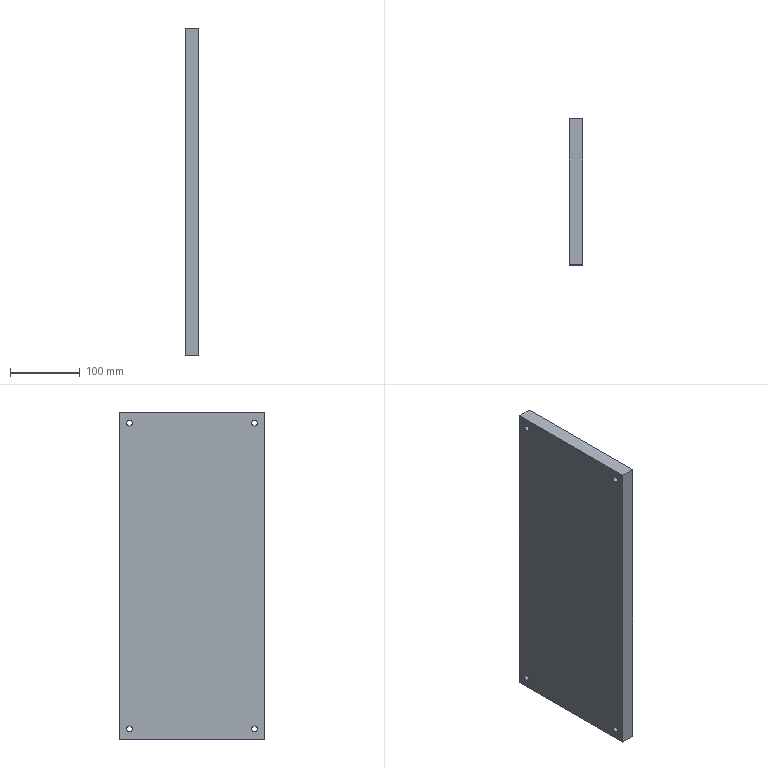Part | STEP file | A14-050 | 1 solid | 14 faces | box 20 x 210 x 470 mm | volume 1969460 mm3 | cylinder 8 | plane 6 | commonest cylinder face diameters 8.5 x8
STEP:
#1=CARTESIAN_POINT('',(0.,0.,0.));
#2=DIRECTION('',(0.,0.,1.));
#3=DIRECTION('',(1.,0.,0.));
#4=AXIS2_PLACEMENT_3D('',#1,#2,#3);
#5=CARTESIAN_POINT('',(-10.,90.,215.75));
#6=VERTEX_POINT('',#5);
#7=CARTESIAN_POINT('',(10.,90.,215.75));
#8=VERTEX_POINT('',#7);
#9=CARTESIAN_POINT('',(-10.,90.,215.75));
#10=DIRECTION('',(1.,0.,0.));
#11=VECTOR('',#10,1.);
#12=LINE('',#9,#11);
#13=CARTESIAN_POINT('',(-10.,90.,220.));
#14=DIRECTION('',(1.,0.,0.));
#15=DIRECTION('',(0.,0.,-1.));
#16=AXIS2_PLACEMENT_3D('',#13,#14,#15);
#17=CYLINDRICAL_SURFACE('',#16,4.25);
#18=CARTESIAN_POINT('',(6.283,0.));
#19=DIRECTION('',(0.,1.));
#20=VECTOR('',#19,1.);
#21=LINE('',#18,#20);
#22=(GEOMETRIC_REPRESENTATION_CONTEXT(2)PARAMETRIC_REPRESENTATION_CONTEXT()REPRESENTATION_CONTEXT('',''));
#23=DEFINITIONAL_REPRESENTATION('',(#21),#22);
#24=PCURVE('',#17,#23);
#25=CARTESIAN_POINT('',(-10.,90.,220.));
#26=DIRECTION('',(1.,0.,0.));
#27=DIRECTION('',(0.,0.,-1.));
#28=AXIS2_PLACEMENT_3D('',#25,#26,#27);
#29=CYLINDRICAL_SURFACE('',#28,4.25);
#30=CARTESIAN_POINT('',(0.,0.));
#31=DIRECTION('',(0.,1.));
#32=VECTOR('',#31,1.);
#33=LINE('',#30,#32);
#34=(GEOMETRIC_REPRESENTATION_CONTEXT(2)PARAMETRIC_REPRESENTATION_CONTEXT()REPRESENTATION_CONTEXT('',''));
#35=DEFINITIONAL_REPRESENTATION('',(#33),#34);
#36=PCURVE('',#29,#35);
#37=SURFACE_CURVE('',#12,(#24,#36),.PCURVE_S1.);
#38=EDGE_CURVE('',#6,#8,#37,.T.);
#39=ORIENTED_EDGE('',*,*,#38,.T.);
#40=CARTESIAN_POINT('',(10.,90.,224.25));
#41=VERTEX_POINT('',#40);
#42=CARTESIAN_POINT('',(10.,90.,220.));
#43=DIRECTION('',(1.,0.,0.));
#44=DIRECTION('',(0.,0.,-1.));
#45=AXIS2_PLACEMENT_3D('',#42,#43,#44);
#46=CIRCLE('',#45,4.25);
#47=CARTESIAN_POINT('',(0.,20.));
#48=DIRECTION('',(1.,0.));
#49=VECTOR('',#48,1.);
#50=LINE('',#47,#49);
#51=(GEOMETRIC_REPRESENTATION_CONTEXT(2)PARAMETRIC_REPRESENTATION_CONTEXT()REPRESENTATION_CONTEXT('',''));
#52=DEFINITIONAL_REPRESENTATION('',(#50),#51);
#53=PCURVE('',#17,#52);
#54=CARTESIAN_POINT('',(10.,0.,0.));
#55=DIRECTION('',(1.,0.,0.));
#56=DIRECTION('',(0.,0.,-1.));
#57=AXIS2_PLACEMENT_3D('',#54,#55,#56);
#58=PLANE('',#57);
#59=CARTESIAN_POINT('',(-220.,90.));
#60=DIRECTION('',(1.,0.));
#61=AXIS2_PLACEMENT_2D('',#59,#60);
#62=CIRCLE('',#61,4.25);
#63=(GEOMETRIC_REPRESENTATION_CONTEXT(2)PARAMETRIC_REPRESENTATION_CONTEXT()REPRESENTATION_CONTEXT('',''));
#64=DEFINITIONAL_REPRESENTATION('',(#62),#63);
#65=PCURVE('',#58,#64);
#66=SURFACE_CURVE('',#46,(#53,#65),.PCURVE_S1.);
#67=EDGE_CURVE('',#41,#8,#66,.T.);
#68=ORIENTED_EDGE('',*,*,#67,.F.);
#69=CARTESIAN_POINT('',(-10.,90.,224.25));
#70=VERTEX_POINT('',#69);
#71=CARTESIAN_POINT('',(-10.,90.,224.25));
#72=DIRECTION('',(1.,0.,0.));
#73=VECTOR('',#72,1.);
#74=LINE('',#71,#73);
#75=CARTESIAN_POINT('',(3.142,0.));
#76=DIRECTION('',(0.,1.));
#77=VECTOR('',#76,1.);
#78=LINE('',#75,#77);
#79=(GEOMETRIC_REPRESENTATION_CONTEXT(2)PARAMETRIC_REPRESENTATION_CONTEXT()REPRESENTATION_CONTEXT('',''));
#80=DEFINITIONAL_REPRESENTATION('',(#78),#79);
#81=PCURVE('',#17,#80);
#82=CARTESIAN_POINT('',(3.142,0.));
#83=DIRECTION('',(0.,1.));
#84=VECTOR('',#83,1.);
#85=LINE('',#82,#84);
#86=(GEOMETRIC_REPRESENTATION_CONTEXT(2)PARAMETRIC_REPRESENTATION_CONTEXT()REPRESENTATION_CONTEXT('',''));
#87=DEFINITIONAL_REPRESENTATION('',(#85),#86);
#88=PCURVE('',#29,#87);
#89=SURFACE_CURVE('',#74,(#81,#88),.PCURVE_S1.);
#90=EDGE_CURVE('',#70,#41,#89,.T.);
#91=ORIENTED_EDGE('',*,*,#90,.F.);
#92=CARTESIAN_POINT('',(-10.,90.,220.));
#93=DIRECTION('',(1.,0.,0.));
#94=DIRECTION('',(0.,0.,-1.));
#95=AXIS2_PLACEMENT_3D('',#92,#93,#94);
#96=CIRCLE('',#95,4.25);
#97=CARTESIAN_POINT('',(0.,0.));
#98=DIRECTION('',(1.,0.));
#99=VECTOR('',#98,1.);
#100=LINE('',#97,#99);
#101=(GEOMETRIC_REPRESENTATION_CONTEXT(2)PARAMETRIC_REPRESENTATION_CONTEXT()REPRESENTATION_CONTEXT('',''));
#102=DEFINITIONAL_REPRESENTATION('',(#100),#101);
#103=PCURVE('',#17,#102);
#104=CARTESIAN_POINT('',(-10.,0.,0.));
#105=DIRECTION('',(1.,0.,0.));
#106=DIRECTION('',(0.,0.,-1.));
#107=AXIS2_PLACEMENT_3D('',#104,#105,#106);
#108=PLANE('',#107);
#109=CARTESIAN_POINT('',(-220.,90.));
#110=DIRECTION('',(1.,0.));
#111=AXIS2_PLACEMENT_2D('',#109,#110);
#112=CIRCLE('',#111,4.25);
#113=(GEOMETRIC_REPRESENTATION_CONTEXT(2)PARAMETRIC_REPRESENTATION_CONTEXT()REPRESENTATION_CONTEXT('',''));
#114=DEFINITIONAL_REPRESENTATION('',(#112),#113);
#115=PCURVE('',#108,#114);
#116=SURFACE_CURVE('',#96,(#103,#115),.PCURVE_S1.);
#117=EDGE_CURVE('',#70,#6,#116,.T.);
#118=ORIENTED_EDGE('',*,*,#117,.T.);
#119=EDGE_LOOP('',(#39,#68,#91,#118));
#120=FACE_BOUND('',#119,.F.);
#121=ADVANCED_FACE('',(#120),#17,.F.);
#122=CARTESIAN_POINT('',(-10.,-90.,215.75));
#123=VERTEX_POINT('',#122);
#124=CARTESIAN_POINT('',(10.,-90.,215.75));
#125=VERTEX_POINT('',#124);
#126=CARTESIAN_POINT('',(-10.,-90.,215.75));
#127=DIRECTION('',(1.,0.,0.));
#128=VECTOR('',#127,1.);
#129=LINE('',#126,#128);
#130=CARTESIAN_POINT('',(-10.,-90.,220.));
#131=DIRECTION('',(1.,0.,0.));
#132=DIRECTION('',(0.,0.,-1.));
#133=AXIS2_PLACEMENT_3D('',#130,#131,#132);
#134=CYLINDRICAL_SURFACE('',#133,4.25);
#135=CARTESIAN_POINT('',(6.283,0.));
#136=DIRECTION('',(0.,1.));
#137=VECTOR('',#136,1.);
#138=LINE('',#135,#137);
#139=(GEOMETRIC_REPRESENTATION_CONTEXT(2)PARAMETRIC_REPRESENTATION_CONTEXT()REPRESENTATION_CONTEXT('',''));
#140=DEFINITIONAL_REPRESENTATION('',(#138),#139);
#141=PCURVE('',#134,#140);
#142=CARTESIAN_POINT('',(-10.,-90.,220.));
#143=DIRECTION('',(1.,0.,0.));
#144=DIRECTION('',(0.,0.,-1.));
#145=AXIS2_PLACEMENT_3D('',#142,#143,#144);
#146=CYLINDRICAL_SURFACE('',#145,4.25);
#147=CARTESIAN_POINT('',(0.,0.));
#148=DIRECTION('',(0.,1.));
#149=VECTOR('',#148,1.);
#150=LINE('',#147,#149);
#151=(GEOMETRIC_REPRESENTATION_CONTEXT(2)PARAMETRIC_REPRESENTATION_CONTEXT()REPRESENTATION_CONTEXT('',''));
#152=DEFINITIONAL_REPRESENTATION('',(#150),#151);
#153=PCURVE('',#146,#152);
#154=SURFACE_CURVE('',#129,(#141,#153),.PCURVE_S1.);
#155=EDGE_CURVE('',#123,#125,#154,.T.);
#156=ORIENTED_EDGE('',*,*,#155,.T.);
#157=CARTESIAN_POINT('',(10.,-90.,224.25));
#158=VERTEX_POINT('',#157);
#159=CARTESIAN_POINT('',(10.,-90.,220.));
#160=DIRECTION('',(1.,0.,0.));
#161=DIRECTION('',(0.,0.,-1.));
#162=AXIS2_PLACEMENT_3D('',#159,#160,#161);
#163=CIRCLE('',#162,4.25);
#164=CARTESIAN_POINT('',(0.,20.));
#165=DIRECTION('',(1.,0.));
#166=VECTOR('',#165,1.);
#167=LINE('',#164,#166);
#168=(GEOMETRIC_REPRESENTATION_CONTEXT(2)PARAMETRIC_REPRESENTATION_CONTEXT()REPRESENTATION_CONTEXT('',''));
#169=DEFINITIONAL_REPRESENTATION('',(#167),#168);
#170=PCURVE('',#134,#169);
#171=CARTESIAN_POINT('',(-220.,-90.));
#172=DIRECTION('',(1.,0.));
#173=AXIS2_PLACEMENT_2D('',#171,#172);
#174=CIRCLE('',#173,4.25);
#175=(GEOMETRIC_REPRESENTATION_CONTEXT(2)PARAMETRIC_REPRESENTATION_CONTEXT()REPRESENTATION_CONTEXT('',''));
#176=DEFINITIONAL_REPRESENTATION('',(#174),#175);
#177=PCURVE('',#58,#176);
#178=SURFACE_CURVE('',#163,(#170,#177),.PCURVE_S1.);
#179=EDGE_CURVE('',#158,#125,#178,.T.);
#180=ORIENTED_EDGE('',*,*,#179,.F.);
#181=CARTESIAN_POINT('',(-10.,-90.,224.25));
#182=VERTEX_POINT('',#181);
#183=CARTESIAN_POINT('',(-10.,-90.,224.25));
#184=DIRECTION('',(1.,0.,0.));
#185=VECTOR('',#184,1.);
#186=LINE('',#183,#185);
#187=CARTESIAN_POINT('',(3.142,0.));
#188=DIRECTION('',(0.,1.));
#189=VECTOR('',#188,1.);
#190=LINE('',#187,#189);
#191=(GEOMETRIC_REPRESENTATION_CONTEXT(2)PARAMETRIC_REPRESENTATION_CONTEXT()REPRESENTATION_CONTEXT('',''));
#192=DEFINITIONAL_REPRESENTATION('',(#190),#191);
#193=PCURVE('',#134,#192);
#194=CARTESIAN_POINT('',(3.142,0.));
#195=DIRECTION('',(0.,1.));
#196=VECTOR('',#195,1.);
#197=LINE('',#194,#196);
#198=(GEOMETRIC_REPRESENTATION_CONTEXT(2)PARAMETRIC_REPRESENTATION_CONTEXT()REPRESENTATION_CONTEXT('',''));
#199=DEFINITIONAL_REPRESENTATION('',(#197),#198);
#200=PCURVE('',#146,#199);
#201=SURFACE_CURVE('',#186,(#193,#200),.PCURVE_S1.);
#202=EDGE_CURVE('',#182,#158,#201,.T.);
#203=ORIENTED_EDGE('',*,*,#202,.F.);
#204=CARTESIAN_POINT('',(-10.,-90.,220.));
#205=DIRECTION('',(1.,0.,0.));
#206=DIRECTION('',(0.,0.,-1.));
#207=AXIS2_PLACEMENT_3D('',#204,#205,#206);
#208=CIRCLE('',#207,4.25);
#209=CARTESIAN_POINT('',(0.,0.));
#210=DIRECTION('',(1.,0.));
#211=VECTOR('',#210,1.);
#212=LINE('',#209,#211);
#213=(GEOMETRIC_REPRESENTATION_CONTEXT(2)PARAMETRIC_REPRESENTATION_CONTEXT()REPRESENTATION_CONTEXT('',''));
#214=DEFINITIONAL_REPRESENTATION('',(#212),#213);
#215=PCURVE('',#134,#214);
#216=CARTESIAN_POINT('',(-220.,-90.));
#217=DIRECTION('',(1.,0.));
#218=AXIS2_PLACEMENT_2D('',#216,#217);
#219=CIRCLE('',#218,4.25);
#220=(GEOMETRIC_REPRESENTATION_CONTEXT(2)PARAMETRIC_REPRESENTATION_CONTEXT()REPRESENTATION_CONTEXT('',''));
#221=DEFINITIONAL_REPRESENTATION('',(#219),#220);
#222=PCURVE('',#108,#221);
#223=SURFACE_CURVE('',#208,(#215,#222),.PCURVE_S1.);
#224=EDGE_CURVE('',#182,#123,#223,.T.);
#225=ORIENTED_EDGE('',*,*,#224,.T.);
#226=EDGE_LOOP('',(#156,#180,#203,#225));
#227=FACE_BOUND('',#226,.F.);
#228=ADVANCED_FACE('',(#227),#134,.F.);
#229=CARTESIAN_POINT('',(-10.,-90.,-224.25));
#230=VERTEX_POINT('',#229);
#231=CARTESIAN_POINT('',(10.,-90.,-224.25));
#232=VERTEX_POINT('',#231);
#233=CARTESIAN_POINT('',(-10.,-90.,-224.25));
#234=DIRECTION('',(1.,0.,0.));
#235=VECTOR('',#234,1.);
#236=LINE('',#233,#235);
#237=CARTESIAN_POINT('',(-10.,-90.,-220.));
#238=DIRECTION('',(1.,0.,0.));
#239=DIRECTION('',(0.,0.,-1.));
#240=AXIS2_PLACEMENT_3D('',#237,#238,#239);
#241=CYLINDRICAL_SURFACE('',#240,4.25);
#242=CARTESIAN_POINT('',(6.283,0.));
#243=DIRECTION('',(0.,1.));
#244=VECTOR('',#243,1.);
#245=LINE('',#242,#244);
#246=(GEOMETRIC_REPRESENTATION_CONTEXT(2)PARAMETRIC_REPRESENTATION_CONTEXT()REPRESENTATION_CONTEXT('',''));
#247=DEFINITIONAL_REPRESENTATION('',(#245),#246);
#248=PCURVE('',#241,#247);
#249=CARTESIAN_POINT('',(-10.,-90.,-220.));
#250=DIRECTION('',(1.,0.,0.));
#251=DIRECTION('',(0.,0.,-1.));
#252=AXIS2_PLACEMENT_3D('',#249,#250,#251);
#253=CYLINDRICAL_SURFACE('',#252,4.25);
#254=CARTESIAN_POINT('',(0.,0.));
#255=DIRECTION('',(0.,1.));
#256=VECTOR('',#255,1.);
#257=LINE('',#254,#256);
#258=(GEOMETRIC_REPRESENTATION_CONTEXT(2)PARAMETRIC_REPRESENTATION_CONTEXT()REPRESENTATION_CONTEXT('',''));
#259=DEFINITIONAL_REPRESENTATION('',(#257),#258);
#260=PCURVE('',#253,#259);
#261=SURFACE_CURVE('',#236,(#248,#260),.PCURVE_S1.);
#262=EDGE_CURVE('',#230,#232,#261,.T.);
#263=ORIENTED_EDGE('',*,*,#262,.T.);
#264=CARTESIAN_POINT('',(10.,-90.,-215.75));
#265=VERTEX_POINT('',#264);
#266=CARTESIAN_POINT('',(10.,-90.,-220.));
#267=DIRECTION('',(1.,0.,0.));
#268=DIRECTION('',(0.,0.,-1.));
#269=AXIS2_PLACEMENT_3D('',#266,#267,#268);
#270=CIRCLE('',#269,4.25);
#271=CARTESIAN_POINT('',(0.,20.));
#272=DIRECTION('',(1.,0.));
#273=VECTOR('',#272,1.);
#274=LINE('',#271,#273);
#275=(GEOMETRIC_REPRESENTATION_CONTEXT(2)PARAMETRIC_REPRESENTATION_CONTEXT()REPRESENTATION_CONTEXT('',''));
#276=DEFINITIONAL_REPRESENTATION('',(#274),#275);
#277=PCURVE('',#241,#276);
#278=CARTESIAN_POINT('',(220.,-90.));
#279=DIRECTION('',(1.,0.));
#280=AXIS2_PLACEMENT_2D('',#278,#279);
#281=CIRCLE('',#280,4.25);
#282=(GEOMETRIC_REPRESENTATION_CONTEXT(2)PARAMETRIC_REPRESENTATION_CONTEXT()REPRESENTATION_CONTEXT('',''));
#283=DEFINITIONAL_REPRESENTATION('',(#281),#282);
#284=PCURVE('',#58,#283);
#285=SURFACE_CURVE('',#270,(#277,#284),.PCURVE_S1.);
#286=EDGE_CURVE('',#265,#232,#285,.T.);
#287=ORIENTED_EDGE('',*,*,#286,.F.);
#288=CARTESIAN_POINT('',(-10.,-90.,-215.75));
#289=VERTEX_POINT('',#288);
#290=CARTESIAN_POINT('',(-10.,-90.,-215.75));
#291=DIRECTION('',(1.,0.,0.));
#292=VECTOR('',#291,1.);
#293=LINE('',#290,#292);
#294=CARTESIAN_POINT('',(3.142,0.));
#295=DIRECTION('',(0.,1.));
#296=VECTOR('',#295,1.);
#297=LINE('',#294,#296);
#298=(GEOMETRIC_REPRESENTATION_CONTEXT(2)PARAMETRIC_REPRESENTATION_CONTEXT()REPRESENTATION_CONTEXT('',''));
#299=DEFINITIONAL_REPRESENTATION('',(#297),#298);
#300=PCURVE('',#241,#299);
#301=CARTESIAN_POINT('',(3.142,0.));
#302=DIRECTION('',(0.,1.));
#303=VECTOR('',#302,1.);
#304=LINE('',#301,#303);
#305=(GEOMETRIC_REPRESENTATION_CONTEXT(2)PARAMETRIC_REPRESENTATION_CONTEXT()REPRESENTATION_CONTEXT('',''));
#306=DEFINITIONAL_REPRESENTATION('',(#304),#305);
#307=PCURVE('',#253,#306);
#308=SURFACE_CURVE('',#293,(#300,#307),.PCURVE_S1.);
#309=EDGE_CURVE('',#289,#265,#308,.T.);
#310=ORIENTED_EDGE('',*,*,#309,.F.);
#311=CARTESIAN_POINT('',(-10.,-90.,-220.));
#312=DIRECTION('',(1.,0.,0.));
#313=DIRECTION('',(0.,0.,-1.));
#314=AXIS2_PLACEMENT_3D('',#311,#312,#313);
#315=CIRCLE('',#314,4.25);
#316=CARTESIAN_POINT('',(0.,0.));
#317=DIRECTION('',(1.,0.));
#318=VECTOR('',#317,1.);
#319=LINE('',#316,#318);
#320=(GEOMETRIC_REPRESENTATION_CONTEXT(2)PARAMETRIC_REPRESENTATION_CONTEXT()REPRESENTATION_CONTEXT('',''));
#321=DEFINITIONAL_REPRESENTATION('',(#319),#320);
#322=PCURVE('',#241,#321);
#323=CARTESIAN_POINT('',(220.,-90.));
#324=DIRECTION('',(1.,0.));
#325=AXIS2_PLACEMENT_2D('',#323,#324);
#326=CIRCLE('',#325,4.25);
#327=(GEOMETRIC_REPRESENTATION_CONTEXT(2)PARAMETRIC_REPRESENTATION_CONTEXT()REPRESENTATION_CONTEXT('',''));
#328=DEFINITIONAL_REPRESENTATION('',(#326),#327);
#329=PCURVE('',#108,#328);
#330=SURFACE_CURVE('',#315,(#322,#329),.PCURVE_S1.);
#331=EDGE_CURVE('',#289,#230,#330,.T.);
#332=ORIENTED_EDGE('',*,*,#331,.T.);
#333=EDGE_LOOP('',(#263,#287,#310,#332));
#334=FACE_BOUND('',#333,.F.);
#335=ADVANCED_FACE('',(#334),#241,.F.);
#336=CARTESIAN_POINT('',(-10.,90.,-224.25));
#337=VERTEX_POINT('',#336);
#338=CARTESIAN_POINT('',(10.,90.,-224.25));
#339=VERTEX_POINT('',#338);
#340=CARTESIAN_POINT('',(-10.,90.,-224.25));
#341=DIRECTION('',(1.,0.,0.));
#342=VECTOR('',#341,1.);
#343=LINE('',#340,#342);
#344=CARTESIAN_POINT('',(-10.,90.,-220.));
#345=DIRECTION('',(1.,0.,0.));
#346=DIRECTION('',(0.,0.,-1.));
#347=AXIS2_PLACEMENT_3D('',#344,#345,#346);
#348=CYLINDRICAL_SURFACE('',#347,4.25);
#349=CARTESIAN_POINT('',(6.283,0.));
#350=DIRECTION('',(0.,1.));
#351=VECTOR('',#350,1.);
#352=LINE('',#349,#351);
#353=(GEOMETRIC_REPRESENTATION_CONTEXT(2)PARAMETRIC_REPRESENTATION_CONTEXT()REPRESENTATION_CONTEXT('',''));
#354=DEFINITIONAL_REPRESENTATION('',(#352),#353);
#355=PCURVE('',#348,#354);
#356=CARTESIAN_POINT('',(-10.,90.,-220.));
#357=DIRECTION('',(1.,0.,0.));
#358=DIRECTION('',(0.,0.,-1.));
#359=AXIS2_PLACEMENT_3D('',#356,#357,#358);
#360=CYLINDRICAL_SURFACE('',#359,4.25);
#361=CARTESIAN_POINT('',(0.,0.));
#362=DIRECTION('',(0.,1.));
#363=VECTOR('',#362,1.);
#364=LINE('',#361,#363);
#365=(GEOMETRIC_REPRESENTATION_CONTEXT(2)PARAMETRIC_REPRESENTATION_CONTEXT()REPRESENTATION_CONTEXT('',''));
#366=DEFINITIONAL_REPRESENTATION('',(#364),#365);
#367=PCURVE('',#360,#366);
#368=SURFACE_CURVE('',#343,(#355,#367),.PCURVE_S1.);
#369=EDGE_CURVE('',#337,#339,#368,.T.);
#370=ORIENTED_EDGE('',*,*,#369,.T.);
#371=CARTESIAN_POINT('',(10.,90.,-215.75));
#372=VERTEX_POINT('',#371);
#373=CARTESIAN_POINT('',(10.,90.,-220.));
#374=DIRECTION('',(1.,0.,0.));
#375=DIRECTION('',(0.,0.,-1.));
#376=AXIS2_PLACEMENT_3D('',#373,#374,#375);
#377=CIRCLE('',#376,4.25);
#378=CARTESIAN_POINT('',(0.,20.));
#379=DIRECTION('',(1.,0.));
#380=VECTOR('',#379,1.);
#381=LINE('',#378,#380);
#382=(GEOMETRIC_REPRESENTATION_CONTEXT(2)PARAMETRIC_REPRESENTATION_CONTEXT()REPRESENTATION_CONTEXT('',''));
#383=DEFINITIONAL_REPRESENTATION('',(#381),#382);
#384=PCURVE('',#348,#383);
#385=CARTESIAN_POINT('',(220.,90.));
#386=DIRECTION('',(1.,0.));
#387=AXIS2_PLACEMENT_2D('',#385,#386);
#388=CIRCLE('',#387,4.25);
#389=(GEOMETRIC_REPRESENTATION_CONTEXT(2)PARAMETRIC_REPRESENTATION_CONTEXT()REPRESENTATION_CONTEXT('',''));
#390=DEFINITIONAL_REPRESENTATION('',(#388),#389);
#391=PCURVE('',#58,#390);
#392=SURFACE_CURVE('',#377,(#384,#391),.PCURVE_S1.);
#393=EDGE_CURVE('',#372,#339,#392,.T.);
#394=ORIENTED_EDGE('',*,*,#393,.F.);
#395=CARTESIAN_POINT('',(-10.,90.,-215.75));
#396=VERTEX_POINT('',#395);
#397=CARTESIAN_POINT('',(-10.,90.,-215.75));
#398=DIRECTION('',(1.,0.,0.));
#399=VECTOR('',#398,1.);
#400=LINE('',#397,#399);
#401=CARTESIAN_POINT('',(3.142,0.));
#402=DIRECTION('',(0.,1.));
#403=VECTOR('',#402,1.);
#404=LINE('',#401,#403);
#405=(GEOMETRIC_REPRESENTATION_CONTEXT(2)PARAMETRIC_REPRESENTATION_CONTEXT()REPRESENTATION_CONTEXT('',''));
#406=DEFINITIONAL_REPRESENTATION('',(#404),#405);
#407=PCURVE('',#348,#406);
#408=CARTESIAN_POINT('',(3.142,0.));
#409=DIRECTION('',(0.,1.));
#410=VECTOR('',#409,1.);
#411=LINE('',#408,#410);
#412=(GEOMETRIC_REPRESENTATION_CONTEXT(2)PARAMETRIC_REPRESENTATION_CONTEXT()REPRESENTATION_CONTEXT('',''));
#413=DEFINITIONAL_REPRESENTATION('',(#411),#412);
#414=PCURVE('',#360,#413);
#415=SURFACE_CURVE('',#400,(#407,#414),.PCURVE_S1.);
#416=EDGE_CURVE('',#396,#372,#415,.T.);
#417=ORIENTED_EDGE('',*,*,#416,.F.);
#418=CARTESIAN_POINT('',(-10.,90.,-220.));
#419=DIRECTION('',(1.,0.,0.));
#420=DIRECTION('',(0.,0.,-1.));
#421=AXIS2_PLACEMENT_3D('',#418,#419,#420);
#422=CIRCLE('',#421,4.25);
#423=CARTESIAN_POINT('',(0.,0.));
#424=DIRECTION('',(1.,0.));
#425=VECTOR('',#424,1.);
#426=LINE('',#423,#425);
#427=(GEOMETRIC_REPRESENTATION_CONTEXT(2)PARAMETRIC_REPRESENTATION_CONTEXT()REPRESENTATION_CONTEXT('',''));
#428=DEFINITIONAL_REPRESENTATION('',(#426),#427);
#429=PCURVE('',#348,#428);
#430=CARTESIAN_POINT('',(220.,90.));
#431=DIRECTION('',(1.,0.));
#432=AXIS2_PLACEMENT_2D('',#430,#431);
#433=CIRCLE('',#432,4.25);
#434=(GEOMETRIC_REPRESENTATION_CONTEXT(2)PARAMETRIC_REPRESENTATION_CONTEXT()REPRESENTATION_CONTEXT('',''));
#435=DEFINITIONAL_REPRESENTATION('',(#433),#434);
#436=PCURVE('',#108,#435);
#437=SURFACE_CURVE('',#422,(#429,#436),.PCURVE_S1.);
#438=EDGE_CURVE('',#396,#337,#437,.T.);
#439=ORIENTED_EDGE('',*,*,#438,.T.);
#440=EDGE_LOOP('',(#370,#394,#417,#439));
#441=FACE_BOUND('',#440,.F.);
#442=ADVANCED_FACE('',(#441),#348,.F.);
#443=CARTESIAN_POINT('',(-10.,-105.,-235.));
#444=VERTEX_POINT('',#443);
#445=CARTESIAN_POINT('',(-10.,105.,-235.));
#446=VERTEX_POINT('',#445);
#447=CARTESIAN_POINT('',(-10.,105.,-235.));
#448=DIRECTION('',(0.,1.,0.));
#449=VECTOR('',#448,1.);
#450=LINE('',#447,#449);
#451=CARTESIAN_POINT('',(10.,105.,-235.));
#452=DIRECTION('',(0.,0.,1.));
#453=DIRECTION('',(1.,0.,0.));
#454=AXIS2_PLACEMENT_3D('',#451,#452,#453);
#455=PLANE('',#454);
#456=CARTESIAN_POINT('',(-20.,0.));
#457=DIRECTION('',(0.,1.));
#458=VECTOR('',#457,1.);
#459=LINE('',#456,#458);
#460=(GEOMETRIC_REPRESENTATION_CONTEXT(2)PARAMETRIC_REPRESENTATION_CONTEXT()REPRESENTATION_CONTEXT('',''));
#461=DEFINITIONAL_REPRESENTATION('',(#459),#460);
#462=PCURVE('',#455,#461);
#463=CARTESIAN_POINT('',(235.,105.));
#464=DIRECTION('',(0.,1.));
#465=VECTOR('',#464,1.);
#466=LINE('',#463,#465);
#467=(GEOMETRIC_REPRESENTATION_CONTEXT(2)PARAMETRIC_REPRESENTATION_CONTEXT()REPRESENTATION_CONTEXT('',''));
#468=DEFINITIONAL_REPRESENTATION('',(#466),#467);
#469=PCURVE('',#108,#468);
#470=SURFACE_CURVE('',#450,(#462,#469),.PCURVE_S1.);
#471=EDGE_CURVE('',#444,#446,#470,.T.);
#472=ORIENTED_EDGE('',*,*,#471,.T.);
#473=CARTESIAN_POINT('',(10.,105.,-235.));
#474=VERTEX_POINT('',#473);
#475=CARTESIAN_POINT('',(10.,105.,-235.));
#476=DIRECTION('',(-1.,0.,0.));
#477=VECTOR('',#476,1.);
#478=LINE('',#475,#477);
#479=CARTESIAN_POINT('',(0.,0.));
#480=DIRECTION('',(-1.,0.));
#481=VECTOR('',#480,1.);
#482=LINE('',#479,#481);
#483=(GEOMETRIC_REPRESENTATION_CONTEXT(2)PARAMETRIC_REPRESENTATION_CONTEXT()REPRESENTATION_CONTEXT('',''));
#484=DEFINITIONAL_REPRESENTATION('',(#482),#483);
#485=PCURVE('',#455,#484);
#486=CARTESIAN_POINT('',(10.,105.,235.));
#487=DIRECTION('',(0.,-1.,0.));
#488=DIRECTION('',(0.,0.,-1.));
#489=AXIS2_PLACEMENT_3D('',#486,#487,#488);
#490=PLANE('',#489);
#491=CARTESIAN_POINT('',(470.,0.));
#492=DIRECTION('',(0.,-1.));
#493=VECTOR('',#492,1.);
#494=LINE('',#491,#493);
#495=(GEOMETRIC_REPRESENTATION_CONTEXT(2)PARAMETRIC_REPRESENTATION_CONTEXT()REPRESENTATION_CONTEXT('',''));
#496=DEFINITIONAL_REPRESENTATION('',(#494),#495);
#497=PCURVE('',#490,#496);
#498=SURFACE_CURVE('',#478,(#485,#497),.PCURVE_S1.);
#499=EDGE_CURVE('',#474,#446,#498,.T.);
#500=ORIENTED_EDGE('',*,*,#499,.F.);
#501=CARTESIAN_POINT('',(10.,-105.,-235.));
#502=VERTEX_POINT('',#501);
#503=CARTESIAN_POINT('',(10.,105.,-235.));
#504=DIRECTION('',(0.,1.,0.));
#505=VECTOR('',#504,1.);
#506=LINE('',#503,#505);
#507=CARTESIAN_POINT('',(0.,0.));
#508=DIRECTION('',(0.,1.));
#509=VECTOR('',#508,1.);
#510=LINE('',#507,#509);
#511=(GEOMETRIC_REPRESENTATION_CONTEXT(2)PARAMETRIC_REPRESENTATION_CONTEXT()REPRESENTATION_CONTEXT('',''));
#512=DEFINITIONAL_REPRESENTATION('',(#510),#511);
#513=PCURVE('',#455,#512);
#514=CARTESIAN_POINT('',(235.,105.));
#515=DIRECTION('',(0.,1.));
#516=VECTOR('',#515,1.);
#517=LINE('',#514,#516);
#518=(GEOMETRIC_REPRESENTATION_CONTEXT(2)PARAMETRIC_REPRESENTATION_CONTEXT()REPRESENTATION_CONTEXT('',''));
#519=DEFINITIONAL_REPRESENTATION('',(#517),#518);
#520=PCURVE('',#58,#519);
#521=SURFACE_CURVE('',#506,(#513,#520),.PCURVE_S1.);
#522=EDGE_CURVE('',#502,#474,#521,.T.);
#523=ORIENTED_EDGE('',*,*,#522,.F.);
#524=CARTESIAN_POINT('',(10.,-105.,-235.));
#525=DIRECTION('',(-1.,0.,0.));
#526=VECTOR('',#525,1.);
#527=LINE('',#524,#526);
#528=CARTESIAN_POINT('',(0.,-210.));
#529=DIRECTION('',(-1.,0.));
#530=VECTOR('',#529,1.);
#531=LINE('',#528,#530);
#532=(GEOMETRIC_REPRESENTATION_CONTEXT(2)PARAMETRIC_REPRESENTATION_CONTEXT()REPRESENTATION_CONTEXT('',''));
#533=DEFINITIONAL_REPRESENTATION('',(#531),#532);
#534=PCURVE('',#455,#533);
#535=CARTESIAN_POINT('',(10.,-105.,235.));
#536=DIRECTION('',(0.,1.,0.));
#537=DIRECTION('',(0.,0.,1.));
#538=AXIS2_PLACEMENT_3D('',#535,#536,#537);
#539=PLANE('',#538);
#540=CARTESIAN_POINT('',(-470.,0.));
#541=DIRECTION('',(0.,-1.));
#542=VECTOR('',#541,1.);
#543=LINE('',#540,#542);
#544=(GEOMETRIC_REPRESENTATION_CONTEXT(2)PARAMETRIC_REPRESENTATION_CONTEXT()REPRESENTATION_CONTEXT('',''));
#545=DEFINITIONAL_REPRESENTATION('',(#543),#544);
#546=PCURVE('',#539,#545);
#547=SURFACE_CURVE('',#527,(#534,#546),.PCURVE_S1.);
#548=EDGE_CURVE('',#502,#444,#547,.T.);
#549=ORIENTED_EDGE('',*,*,#548,.T.);
#550=EDGE_LOOP('',(#472,#500,#523,#549));
#551=FACE_BOUND('',#550,.T.);
#552=ADVANCED_FACE('',(#551),#455,.F.);
#553=CARTESIAN_POINT('',(-10.,105.,235.));
#554=VERTEX_POINT('',#553);
#555=CARTESIAN_POINT('',(-10.,105.,235.));
#556=DIRECTION('',(0.,0.,1.));
#557=VECTOR('',#556,1.);
#558=LINE('',#555,#557);
#559=CARTESIAN_POINT('',(0.,-20.));
#560=DIRECTION('',(-1.,0.));
#561=VECTOR('',#560,1.);
#562=LINE('',#559,#561);
#563=(GEOMETRIC_REPRESENTATION_CONTEXT(2)PARAMETRIC_REPRESENTATION_CONTEXT()REPRESENTATION_CONTEXT('',''));
#564=DEFINITIONAL_REPRESENTATION('',(#562),#563);
#565=PCURVE('',#490,#564);
#566=CARTESIAN_POINT('',(-235.,105.));
#567=DIRECTION('',(-1.,0.));
#568=VECTOR('',#567,1.);
#569=LINE('',#566,#568);
#570=(GEOMETRIC_REPRESENTATION_CONTEXT(2)PARAMETRIC_REPRESENTATION_CONTEXT()REPRESENTATION_CONTEXT('',''));
#571=DEFINITIONAL_REPRESENTATION('',(#569),#570);
#572=PCURVE('',#108,#571);
#573=SURFACE_CURVE('',#558,(#565,#572),.PCURVE_S1.);
#574=EDGE_CURVE('',#446,#554,#573,.T.);
#575=ORIENTED_EDGE('',*,*,#574,.T.);
#576=CARTESIAN_POINT('',(10.,105.,235.));
#577=VERTEX_POINT('',#576);
#578=CARTESIAN_POINT('',(10.,105.,235.));
#579=DIRECTION('',(-1.,0.,0.));
#580=VECTOR('',#579,1.);
#581=LINE('',#578,#580);
#582=CARTESIAN_POINT('',(0.,0.));
#583=DIRECTION('',(0.,-1.));
#584=VECTOR('',#583,1.);
#585=LINE('',#582,#584);
#586=(GEOMETRIC_REPRESENTATION_CONTEXT(2)PARAMETRIC_REPRESENTATION_CONTEXT()REPRESENTATION_CONTEXT('',''));
#587=DEFINITIONAL_REPRESENTATION('',(#585),#586);
#588=PCURVE('',#490,#587);
#589=CARTESIAN_POINT('',(10.,105.,235.));
#590=DIRECTION('',(0.,0.,-1.));
#591=DIRECTION('',(-1.,0.,0.));
#592=AXIS2_PLACEMENT_3D('',#589,#590,#591);
#593=PLANE('',#592);
#594=CARTESIAN_POINT('',(0.,0.));
#595=DIRECTION('',(1.,0.));
#596=VECTOR('',#595,1.);
#597=LINE('',#594,#596);
#598=(GEOMETRIC_REPRESENTATION_CONTEXT(2)PARAMETRIC_REPRESENTATION_CONTEXT()REPRESENTATION_CONTEXT('',''));
#599=DEFINITIONAL_REPRESENTATION('',(#597),#598);
#600=PCURVE('',#593,#599);
#601=SURFACE_CURVE('',#581,(#588,#600),.PCURVE_S1.);
#602=EDGE_CURVE('',#577,#554,#601,.T.);
#603=ORIENTED_EDGE('',*,*,#602,.F.);
#604=CARTESIAN_POINT('',(10.,105.,235.));
#605=DIRECTION('',(0.,0.,1.));
#606=VECTOR('',#605,1.);
#607=LINE('',#604,#606);
#608=CARTESIAN_POINT('',(0.,0.));
#609=DIRECTION('',(-1.,0.));
#610=VECTOR('',#609,1.);
#611=LINE('',#608,#610);
#612=(GEOMETRIC_REPRESENTATION_CONTEXT(2)PARAMETRIC_REPRESENTATION_CONTEXT()REPRESENTATION_CONTEXT('',''));
#613=DEFINITIONAL_REPRESENTATION('',(#611),#612);
#614=PCURVE('',#490,#613);
#615=CARTESIAN_POINT('',(-235.,105.));
#616=DIRECTION('',(-1.,0.));
#617=VECTOR('',#616,1.);
#618=LINE('',#615,#617);
#619=(GEOMETRIC_REPRESENTATION_CONTEXT(2)PARAMETRIC_REPRESENTATION_CONTEXT()REPRESENTATION_CONTEXT('',''));
#620=DEFINITIONAL_REPRESENTATION('',(#618),#619);
#621=PCURVE('',#58,#620);
#622=SURFACE_CURVE('',#607,(#614,#621),.PCURVE_S1.);
#623=EDGE_CURVE('',#474,#577,#622,.T.);
#624=ORIENTED_EDGE('',*,*,#623,.F.);
#625=ORIENTED_EDGE('',*,*,#499,.T.);
#626=EDGE_LOOP('',(#575,#603,#624,#625));
#627=FACE_BOUND('',#626,.T.);
#628=ADVANCED_FACE('',(#627),#490,.F.);
#629=CARTESIAN_POINT('',(-10.,-105.,235.));
#630=VERTEX_POINT('',#629);
#631=CARTESIAN_POINT('',(-10.,105.,235.));
#632=DIRECTION('',(0.,-1.,0.));
#633=VECTOR('',#632,1.);
#634=LINE('',#631,#633);
#635=CARTESIAN_POINT('',(20.,0.));
#636=DIRECTION('',(0.,-1.));
#637=VECTOR('',#636,1.);
#638=LINE('',#635,#637);
#639=(GEOMETRIC_REPRESENTATION_CONTEXT(2)PARAMETRIC_REPRESENTATION_CONTEXT()REPRESENTATION_CONTEXT('',''));
#640=DEFINITIONAL_REPRESENTATION('',(#638),#639);
#641=PCURVE('',#593,#640);
#642=CARTESIAN_POINT('',(-235.,105.));
#643=DIRECTION('',(0.,-1.));
#644=VECTOR('',#643,1.);
#645=LINE('',#642,#644);
#646=(GEOMETRIC_REPRESENTATION_CONTEXT(2)PARAMETRIC_REPRESENTATION_CONTEXT()REPRESENTATION_CONTEXT('',''));
#647=DEFINITIONAL_REPRESENTATION('',(#645),#646);
#648=PCURVE('',#108,#647);
#649=SURFACE_CURVE('',#634,(#641,#648),.PCURVE_S1.);
#650=EDGE_CURVE('',#554,#630,#649,.T.);
#651=ORIENTED_EDGE('',*,*,#650,.T.);
#652=CARTESIAN_POINT('',(10.,-105.,235.));
#653=VERTEX_POINT('',#652);
#654=CARTESIAN_POINT('',(10.,-105.,235.));
#655=DIRECTION('',(-1.,0.,0.));
#656=VECTOR('',#655,1.);
#657=LINE('',#654,#656);
#658=CARTESIAN_POINT('',(0.,-210.));
#659=DIRECTION('',(1.,0.));
#660=VECTOR('',#659,1.);
#661=LINE('',#658,#660);
#662=(GEOMETRIC_REPRESENTATION_CONTEXT(2)PARAMETRIC_REPRESENTATION_CONTEXT()REPRESENTATION_CONTEXT('',''));
#663=DEFINITIONAL_REPRESENTATION('',(#661),#662);
#664=PCURVE('',#593,#663);
#665=CARTESIAN_POINT('',(0.,0.));
#666=DIRECTION('',(0.,-1.));
#667=VECTOR('',#666,1.);
#668=LINE('',#665,#667);
#669=(GEOMETRIC_REPRESENTATION_CONTEXT(2)PARAMETRIC_REPRESENTATION_CONTEXT()REPRESENTATION_CONTEXT('',''));
#670=DEFINITIONAL_REPRESENTATION('',(#668),#669);
#671=PCURVE('',#539,#670);
#672=SURFACE_CURVE('',#657,(#664,#671),.PCURVE_S1.);
#673=EDGE_CURVE('',#653,#630,#672,.T.);
#674=ORIENTED_EDGE('',*,*,#673,.F.);
#675=CARTESIAN_POINT('',(10.,105.,235.));
#676=DIRECTION('',(0.,-1.,0.));
#677=VECTOR('',#676,1.);
#678=LINE('',#675,#677);
#679=CARTESIAN_POINT('',(0.,0.));
#680=DIRECTION('',(0.,-1.));
#681=VECTOR('',#680,1.);
#682=LINE('',#679,#681);
#683=(GEOMETRIC_REPRESENTATION_CONTEXT(2)PARAMETRIC_REPRESENTATION_CONTEXT()REPRESENTATION_CONTEXT('',''));
#684=DEFINITIONAL_REPRESENTATION('',(#682),#683);
#685=PCURVE('',#593,#684);
#686=CARTESIAN_POINT('',(-235.,105.));
#687=DIRECTION('',(0.,-1.));
#688=VECTOR('',#687,1.);
#689=LINE('',#686,#688);
#690=(GEOMETRIC_REPRESENTATION_CONTEXT(2)PARAMETRIC_REPRESENTATION_CONTEXT()REPRESENTATION_CONTEXT('',''));
#691=DEFINITIONAL_REPRESENTATION('',(#689),#690);
#692=PCURVE('',#58,#691);
#693=SURFACE_CURVE('',#678,(#685,#692),.PCURVE_S1.);
#694=EDGE_CURVE('',#577,#653,#693,.T.);
#695=ORIENTED_EDGE('',*,*,#694,.F.);
#696=ORIENTED_EDGE('',*,*,#602,.T.);
#697=EDGE_LOOP('',(#651,#674,#695,#696));
#698=FACE_BOUND('',#697,.T.);
#699=ADVANCED_FACE('',(#698),#593,.F.);
#700=CARTESIAN_POINT('',(-10.,-105.,235.));
#701=DIRECTION('',(0.,0.,-1.));
#702=VECTOR('',#701,1.);
#703=LINE('',#700,#702);
#704=CARTESIAN_POINT('',(0.,-20.));
#705=DIRECTION('',(-1.,0.));
#706=VECTOR('',#705,1.);
#707=LINE('',#704,#706);
#708=(GEOMETRIC_REPRESENTATION_CONTEXT(2)PARAMETRIC_REPRESENTATION_CONTEXT()REPRESENTATION_CONTEXT('',''));
#709=DEFINITIONAL_REPRESENTATION('',(#707),#708);
#710=PCURVE('',#539,#709);
#711=CARTESIAN_POINT('',(-235.,-105.));
#712=DIRECTION('',(1.,0.));
#713=VECTOR('',#712,1.);
#714=LINE('',#711,#713);
#715=(GEOMETRIC_REPRESENTATION_CONTEXT(2)PARAMETRIC_REPRESENTATION_CONTEXT()REPRESENTATION_CONTEXT('',''));
#716=DEFINITIONAL_REPRESENTATION('',(#714),#715);
#717=PCURVE('',#108,#716);
#718=SURFACE_CURVE('',#703,(#710,#717),.PCURVE_S1.);
#719=EDGE_CURVE('',#630,#444,#718,.T.);
#720=ORIENTED_EDGE('',*,*,#719,.T.);
#721=ORIENTED_EDGE('',*,*,#548,.F.);
#722=CARTESIAN_POINT('',(10.,-105.,235.));
#723=DIRECTION('',(0.,0.,-1.));
#724=VECTOR('',#723,1.);
#725=LINE('',#722,#724);
#726=CARTESIAN_POINT('',(0.,0.));
#727=DIRECTION('',(-1.,0.));
#728=VECTOR('',#727,1.);
#729=LINE('',#726,#728);
#730=(GEOMETRIC_REPRESENTATION_CONTEXT(2)PARAMETRIC_REPRESENTATION_CONTEXT()REPRESENTATION_CONTEXT('',''));
#731=DEFINITIONAL_REPRESENTATION('',(#729),#730);
#732=PCURVE('',#539,#731);
#733=CARTESIAN_POINT('',(-235.,-105.));
#734=DIRECTION('',(1.,0.));
#735=VECTOR('',#734,1.);
#736=LINE('',#733,#735);
#737=(GEOMETRIC_REPRESENTATION_CONTEXT(2)PARAMETRIC_REPRESENTATION_CONTEXT()REPRESENTATION_CONTEXT('',''));
#738=DEFINITIONAL_REPRESENTATION('',(#736),#737);
#739=PCURVE('',#58,#738);
#740=SURFACE_CURVE('',#725,(#732,#739),.PCURVE_S1.);
#741=EDGE_CURVE('',#653,#502,#740,.T.);
#742=ORIENTED_EDGE('',*,*,#741,.F.);
#743=ORIENTED_EDGE('',*,*,#673,.T.);
#744=EDGE_LOOP('',(#720,#721,#742,#743));
#745=FACE_BOUND('',#744,.T.);
#746=ADVANCED_FACE('',(#745),#539,.F.);
#747=CARTESIAN_POINT('',(10.,90.,220.));
#748=DIRECTION('',(1.,0.,0.));
#749=DIRECTION('',(0.,0.,-1.));
#750=AXIS2_PLACEMENT_3D('',#747,#748,#749);
#751=CIRCLE('',#750,4.25);
#752=CARTESIAN_POINT('',(-220.,90.));
#753=DIRECTION('',(1.,0.));
#754=AXIS2_PLACEMENT_2D('',#752,#753);
#755=CIRCLE('',#754,4.25);
#756=(GEOMETRIC_REPRESENTATION_CONTEXT(2)PARAMETRIC_REPRESENTATION_CONTEXT()REPRESENTATION_CONTEXT('',''));
#757=DEFINITIONAL_REPRESENTATION('',(#755),#756);
#758=PCURVE('',#58,#757);
#759=CARTESIAN_POINT('',(0.,20.));
#760=DIRECTION('',(1.,0.));
#761=VECTOR('',#760,1.);
#762=LINE('',#759,#761);
#763=(GEOMETRIC_REPRESENTATION_CONTEXT(2)PARAMETRIC_REPRESENTATION_CONTEXT()REPRESENTATION_CONTEXT('',''));
#764=DEFINITIONAL_REPRESENTATION('',(#762),#763);
#765=PCURVE('',#29,#764);
#766=SURFACE_CURVE('',#751,(#758,#765),.PCURVE_S1.);
#767=EDGE_CURVE('',#8,#41,#766,.T.);
#768=ORIENTED_EDGE('',*,*,#767,.F.);
#769=ORIENTED_EDGE('',*,*,#67,.F.);
#770=EDGE_LOOP('',(#768,#769));
#771=FACE_BOUND('',#770,.T.);
#772=CARTESIAN_POINT('',(10.,-90.,220.));
#773=DIRECTION('',(1.,0.,0.));
#774=DIRECTION('',(0.,0.,-1.));
#775=AXIS2_PLACEMENT_3D('',#772,#773,#774);
#776=CIRCLE('',#775,4.25);
#777=CARTESIAN_POINT('',(-220.,-90.));
#778=DIRECTION('',(1.,0.));
#779=AXIS2_PLACEMENT_2D('',#777,#778);
#780=CIRCLE('',#779,4.25);
#781=(GEOMETRIC_REPRESENTATION_CONTEXT(2)PARAMETRIC_REPRESENTATION_CONTEXT()REPRESENTATION_CONTEXT('',''));
#782=DEFINITIONAL_REPRESENTATION('',(#780),#781);
#783=PCURVE('',#58,#782);
#784=CARTESIAN_POINT('',(0.,20.));
#785=DIRECTION('',(1.,0.));
#786=VECTOR('',#785,1.);
#787=LINE('',#784,#786);
#788=(GEOMETRIC_REPRESENTATION_CONTEXT(2)PARAMETRIC_REPRESENTATION_CONTEXT()REPRESENTATION_CONTEXT('',''));
#789=DEFINITIONAL_REPRESENTATION('',(#787),#788);
#790=PCURVE('',#146,#789);
#791=SURFACE_CURVE('',#776,(#783,#790),.PCURVE_S1.);
#792=EDGE_CURVE('',#125,#158,#791,.T.);
#793=ORIENTED_EDGE('',*,*,#792,.F.);
#794=ORIENTED_EDGE('',*,*,#179,.F.);
#795=EDGE_LOOP('',(#793,#794));
#796=FACE_BOUND('',#795,.T.);
#797=CARTESIAN_POINT('',(10.,-90.,-220.));
#798=DIRECTION('',(1.,0.,0.));
#799=DIRECTION('',(0.,0.,-1.));
#800=AXIS2_PLACEMENT_3D('',#797,#798,#799);
#801=CIRCLE('',#800,4.25);
#802=CARTESIAN_POINT('',(220.,-90.));
#803=DIRECTION('',(1.,0.));
#804=AXIS2_PLACEMENT_2D('',#802,#803);
#805=CIRCLE('',#804,4.25);
#806=(GEOMETRIC_REPRESENTATION_CONTEXT(2)PARAMETRIC_REPRESENTATION_CONTEXT()REPRESENTATION_CONTEXT('',''));
#807=DEFINITIONAL_REPRESENTATION('',(#805),#806);
#808=PCURVE('',#58,#807);
#809=CARTESIAN_POINT('',(0.,20.));
#810=DIRECTION('',(1.,0.));
#811=VECTOR('',#810,1.);
#812=LINE('',#809,#811);
#813=(GEOMETRIC_REPRESENTATION_CONTEXT(2)PARAMETRIC_REPRESENTATION_CONTEXT()REPRESENTATION_CONTEXT('',''));
#814=DEFINITIONAL_REPRESENTATION('',(#812),#813);
#815=PCURVE('',#253,#814);
#816=SURFACE_CURVE('',#801,(#808,#815),.PCURVE_S1.);
#817=EDGE_CURVE('',#232,#265,#816,.T.);
#818=ORIENTED_EDGE('',*,*,#817,.F.);
#819=ORIENTED_EDGE('',*,*,#286,.F.);
#820=EDGE_LOOP('',(#818,#819));
#821=FACE_BOUND('',#820,.T.);
#822=CARTESIAN_POINT('',(10.,90.,-220.));
#823=DIRECTION('',(1.,0.,0.));
#824=DIRECTION('',(0.,0.,-1.));
#825=AXIS2_PLACEMENT_3D('',#822,#823,#824);
#826=CIRCLE('',#825,4.25);
#827=CARTESIAN_POINT('',(220.,90.));
#828=DIRECTION('',(1.,0.));
#829=AXIS2_PLACEMENT_2D('',#827,#828);
#830=CIRCLE('',#829,4.25);
#831=(GEOMETRIC_REPRESENTATION_CONTEXT(2)PARAMETRIC_REPRESENTATION_CONTEXT()REPRESENTATION_CONTEXT('',''));
#832=DEFINITIONAL_REPRESENTATION('',(#830),#831);
#833=PCURVE('',#58,#832);
#834=CARTESIAN_POINT('',(0.,20.));
#835=DIRECTION('',(1.,0.));
#836=VECTOR('',#835,1.);
#837=LINE('',#834,#836);
#838=(GEOMETRIC_REPRESENTATION_CONTEXT(2)PARAMETRIC_REPRESENTATION_CONTEXT()REPRESENTATION_CONTEXT('',''));
#839=DEFINITIONAL_REPRESENTATION('',(#837),#838);
#840=PCURVE('',#360,#839);
#841=SURFACE_CURVE('',#826,(#833,#840),.PCURVE_S1.);
#842=EDGE_CURVE('',#339,#372,#841,.T.);
#843=ORIENTED_EDGE('',*,*,#842,.F.);
#844=ORIENTED_EDGE('',*,*,#393,.F.);
#845=EDGE_LOOP('',(#843,#844));
#846=FACE_BOUND('',#845,.T.);
#847=ORIENTED_EDGE('',*,*,#522,.T.);
#848=ORIENTED_EDGE('',*,*,#623,.T.);
#849=ORIENTED_EDGE('',*,*,#694,.T.);
#850=ORIENTED_EDGE('',*,*,#741,.T.);
#851=EDGE_LOOP('',(#847,#848,#849,#850));
#852=FACE_BOUND('',#851,.T.);
#853=ADVANCED_FACE('',(#771,#796,#821,#846,#852),#58,.T.);
#854=CARTESIAN_POINT('',(-10.,90.,220.));
#855=DIRECTION('',(1.,0.,0.));
#856=DIRECTION('',(0.,0.,-1.));
#857=AXIS2_PLACEMENT_3D('',#854,#855,#856);
#858=CIRCLE('',#857,4.25);
#859=CARTESIAN_POINT('',(-220.,90.));
#860=DIRECTION('',(1.,0.));
#861=AXIS2_PLACEMENT_2D('',#859,#860);
#862=CIRCLE('',#861,4.25);
#863=(GEOMETRIC_REPRESENTATION_CONTEXT(2)PARAMETRIC_REPRESENTATION_CONTEXT()REPRESENTATION_CONTEXT('',''));
#864=DEFINITIONAL_REPRESENTATION('',(#862),#863);
#865=PCURVE('',#108,#864);
#866=CARTESIAN_POINT('',(0.,0.));
#867=DIRECTION('',(1.,0.));
#868=VECTOR('',#867,1.);
#869=LINE('',#866,#868);
#870=(GEOMETRIC_REPRESENTATION_CONTEXT(2)PARAMETRIC_REPRESENTATION_CONTEXT()REPRESENTATION_CONTEXT('',''));
#871=DEFINITIONAL_REPRESENTATION('',(#869),#870);
#872=PCURVE('',#29,#871);
#873=SURFACE_CURVE('',#858,(#865,#872),.PCURVE_S1.);
#874=EDGE_CURVE('',#6,#70,#873,.T.);
#875=ORIENTED_EDGE('',*,*,#874,.T.);
#876=ORIENTED_EDGE('',*,*,#117,.T.);
#877=EDGE_LOOP('',(#875,#876));
#878=FACE_BOUND('',#877,.T.);
#879=CARTESIAN_POINT('',(-10.,-90.,220.));
#880=DIRECTION('',(1.,0.,0.));
#881=DIRECTION('',(0.,0.,-1.));
#882=AXIS2_PLACEMENT_3D('',#879,#880,#881);
#883=CIRCLE('',#882,4.25);
#884=CARTESIAN_POINT('',(-220.,-90.));
#885=DIRECTION('',(1.,0.));
#886=AXIS2_PLACEMENT_2D('',#884,#885);
#887=CIRCLE('',#886,4.25);
#888=(GEOMETRIC_REPRESENTATION_CONTEXT(2)PARAMETRIC_REPRESENTATION_CONTEXT()REPRESENTATION_CONTEXT('',''));
#889=DEFINITIONAL_REPRESENTATION('',(#887),#888);
#890=PCURVE('',#108,#889);
#891=CARTESIAN_POINT('',(0.,0.));
#892=DIRECTION('',(1.,0.));
#893=VECTOR('',#892,1.);
#894=LINE('',#891,#893);
#895=(GEOMETRIC_REPRESENTATION_CONTEXT(2)PARAMETRIC_REPRESENTATION_CONTEXT()REPRESENTATION_CONTEXT('',''));
#896=DEFINITIONAL_REPRESENTATION('',(#894),#895);
#897=PCURVE('',#146,#896);
#898=SURFACE_CURVE('',#883,(#890,#897),.PCURVE_S1.);
#899=EDGE_CURVE('',#123,#182,#898,.T.);
#900=ORIENTED_EDGE('',*,*,#899,.T.);
#901=ORIENTED_EDGE('',*,*,#224,.T.);
#902=EDGE_LOOP('',(#900,#901));
#903=FACE_BOUND('',#902,.T.);
#904=CARTESIAN_POINT('',(-10.,-90.,-220.));
#905=DIRECTION('',(1.,0.,0.));
#906=DIRECTION('',(0.,0.,-1.));
#907=AXIS2_PLACEMENT_3D('',#904,#905,#906);
#908=CIRCLE('',#907,4.25);
#909=CARTESIAN_POINT('',(220.,-90.));
#910=DIRECTION('',(1.,0.));
#911=AXIS2_PLACEMENT_2D('',#909,#910);
#912=CIRCLE('',#911,4.25);
#913=(GEOMETRIC_REPRESENTATION_CONTEXT(2)PARAMETRIC_REPRESENTATION_CONTEXT()REPRESENTATION_CONTEXT('',''));
#914=DEFINITIONAL_REPRESENTATION('',(#912),#913);
#915=PCURVE('',#108,#914);
#916=CARTESIAN_POINT('',(0.,0.));
#917=DIRECTION('',(1.,0.));
#918=VECTOR('',#917,1.);
#919=LINE('',#916,#918);
#920=(GEOMETRIC_REPRESENTATION_CONTEXT(2)PARAMETRIC_REPRESENTATION_CONTEXT()REPRESENTATION_CONTEXT('',''));
#921=DEFINITIONAL_REPRESENTATION('',(#919),#920);
#922=PCURVE('',#253,#921);
#923=SURFACE_CURVE('',#908,(#915,#922),.PCURVE_S1.);
#924=EDGE_CURVE('',#230,#289,#923,.T.);
#925=ORIENTED_EDGE('',*,*,#924,.T.);
#926=ORIENTED_EDGE('',*,*,#331,.T.);
#927=EDGE_LOOP('',(#925,#926));
#928=FACE_BOUND('',#927,.T.);
#929=CARTESIAN_POINT('',(-10.,90.,-220.));
#930=DIRECTION('',(1.,0.,0.));
#931=DIRECTION('',(0.,0.,-1.));
#932=AXIS2_PLACEMENT_3D('',#929,#930,#931);
#933=CIRCLE('',#932,4.25);
#934=CARTESIAN_POINT('',(220.,90.));
#935=DIRECTION('',(1.,0.));
#936=AXIS2_PLACEMENT_2D('',#934,#935);
#937=CIRCLE('',#936,4.25);
#938=(GEOMETRIC_REPRESENTATION_CONTEXT(2)PARAMETRIC_REPRESENTATION_CONTEXT()REPRESENTATION_CONTEXT('',''));
#939=DEFINITIONAL_REPRESENTATION('',(#937),#938);
#940=PCURVE('',#108,#939);
#941=CARTESIAN_POINT('',(0.,0.));
#942=DIRECTION('',(1.,0.));
#943=VECTOR('',#942,1.);
#944=LINE('',#941,#943);
#945=(GEOMETRIC_REPRESENTATION_CONTEXT(2)PARAMETRIC_REPRESENTATION_CONTEXT()REPRESENTATION_CONTEXT('',''));
#946=DEFINITIONAL_REPRESENTATION('',(#944),#945);
#947=PCURVE('',#360,#946);
#948=SURFACE_CURVE('',#933,(#940,#947),.PCURVE_S1.);
#949=EDGE_CURVE('',#337,#396,#948,.T.);
#950=ORIENTED_EDGE('',*,*,#949,.T.);
#951=ORIENTED_EDGE('',*,*,#438,.T.);
#952=EDGE_LOOP('',(#950,#951));
#953=FACE_BOUND('',#952,.T.);
#954=ORIENTED_EDGE('',*,*,#471,.F.);
#955=ORIENTED_EDGE('',*,*,#719,.F.);
#956=ORIENTED_EDGE('',*,*,#650,.F.);
#957=ORIENTED_EDGE('',*,*,#574,.F.);
#958=EDGE_LOOP('',(#954,#955,#956,#957));
#959=FACE_BOUND('',#958,.T.);
#960=ADVANCED_FACE('',(#878,#903,#928,#953,#959),#108,.F.);
#961=ORIENTED_EDGE('',*,*,#842,.F.);
#962=ORIENTED_EDGE('',*,*,#369,.F.);
#963=ORIENTED_EDGE('',*,*,#949,.T.);
#964=ORIENTED_EDGE('',*,*,#416,.T.);
#965=EDGE_LOOP('',(#961,#962,#963,#964));
#966=FACE_BOUND('',#965,.F.);
#967=ADVANCED_FACE('',(#966),#360,.F.);
#968=ORIENTED_EDGE('',*,*,#817,.F.);
#969=ORIENTED_EDGE('',*,*,#262,.F.);
#970=ORIENTED_EDGE('',*,*,#924,.T.);
#971=ORIENTED_EDGE('',*,*,#309,.T.);
#972=EDGE_LOOP('',(#968,#969,#970,#971));
#973=FACE_BOUND('',#972,.F.);
#974=ADVANCED_FACE('',(#973),#253,.F.);
#975=ORIENTED_EDGE('',*,*,#792,.F.);
#976=ORIENTED_EDGE('',*,*,#155,.F.);
#977=ORIENTED_EDGE('',*,*,#899,.T.);
#978=ORIENTED_EDGE('',*,*,#202,.T.);
#979=EDGE_LOOP('',(#975,#976,#977,#978));
#980=FACE_BOUND('',#979,.F.);
#981=ADVANCED_FACE('',(#980),#146,.F.);
#982=ORIENTED_EDGE('',*,*,#767,.F.);
#983=ORIENTED_EDGE('',*,*,#38,.F.);
#984=ORIENTED_EDGE('',*,*,#874,.T.);
#985=ORIENTED_EDGE('',*,*,#90,.T.);
#986=EDGE_LOOP('',(#982,#983,#984,#985));
#987=FACE_BOUND('',#986,.F.);
#988=ADVANCED_FACE('',(#987),#29,.F.);
#989=CLOSED_SHELL('',(#121,#228,#335,#442,#552,#628,#699,#746,#853,#960,#967,#974,#981,#988));
#990=MANIFOLD_SOLID_BREP('',#989);
#991=(LENGTH_UNIT()NAMED_UNIT(*)SI_UNIT(.MILLI.,.METRE.));
#992=UNCERTAINTY_MEASURE_WITH_UNIT(LENGTH_MEASURE(0.0000001),#991,'','');
#993=(NAMED_UNIT(*)PLANE_ANGLE_UNIT()SI_UNIT($,.RADIAN.));
#994=(NAMED_UNIT(*)SI_UNIT($,.STERADIAN.)SOLID_ANGLE_UNIT());
#995=(GEOMETRIC_REPRESENTATION_CONTEXT(3)GLOBAL_UNCERTAINTY_ASSIGNED_CONTEXT((#992))GLOBAL_UNIT_ASSIGNED_CONTEXT((#991,#993,#994))REPRESENTATION_CONTEXT('',''));
#996=ADVANCED_BREP_SHAPE_REPRESENTATION('',(#4,#990),#995);